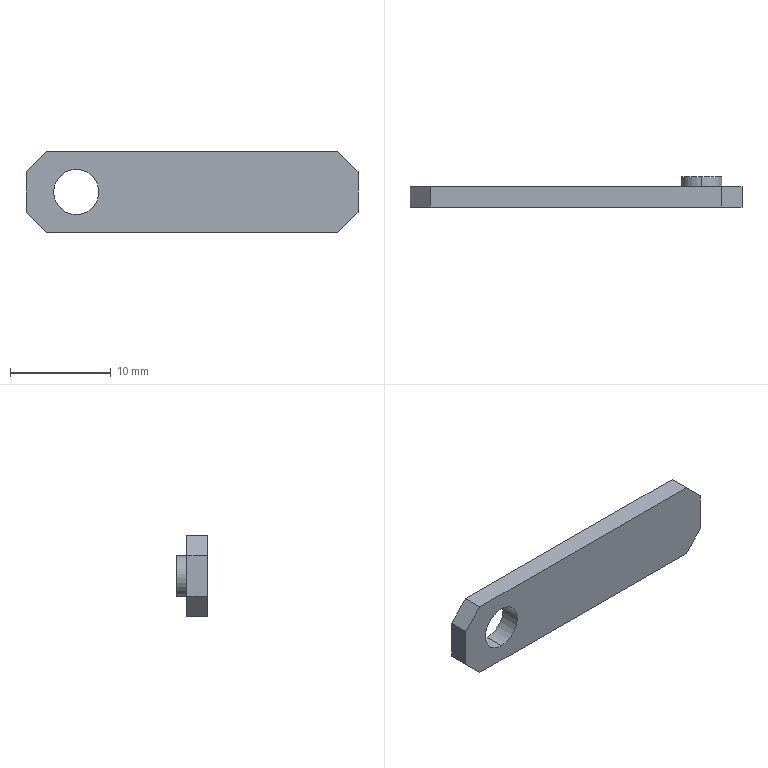Part | SolidWorks | features Chamfer 2, ICE 2, Extrusion 1 | 1 solid | 15 faces | box 33 x 3 x 8 mm | volume 492.758 mm3 | plane 11 | cylinder 4 | commonest cylinder face diameters 4 x2 4.5 x2
STEP:
#1=CARTESIAN_POINT('',(19.307,3.,-1.484));
#2=VERTEX_POINT('',#1);
#3=CARTESIAN_POINT('',(19.307,3.,-5.484));
#4=VERTEX_POINT('',#3);
#5=CARTESIAN_POINT('',(19.307,3.,-3.484));
#6=DIRECTION('',(0.,1.,0.));
#7=DIRECTION('',(0.,0.,1.));
#8=AXIS2_PLACEMENT_3D('',#5,#6,#7);
#9=CIRCLE('',#8,2.);
#10=EDGE_CURVE('',#2,#4,#9,.T.);
#11=ORIENTED_EDGE('',*,*,#10,.F.);
#12=CARTESIAN_POINT('',(19.307,2.,-1.484));
#13=VERTEX_POINT('',#12);
#14=CARTESIAN_POINT('',(19.307,3.,-1.484));
#15=DIRECTION('',(0.,-1.,0.));
#16=VECTOR('',#15,1000.);
#17=LINE('',#14,#16);
#18=EDGE_CURVE('',#2,#13,#17,.T.);
#19=ORIENTED_EDGE('',*,*,#18,.T.);
#20=CARTESIAN_POINT('',(19.307,2.,-5.484));
#21=VERTEX_POINT('',#20);
#22=CARTESIAN_POINT('',(19.307,2.,-3.484));
#23=DIRECTION('',(0.,1.,0.));
#24=DIRECTION('',(0.,0.,1.));
#25=AXIS2_PLACEMENT_3D('',#22,#23,#24);
#26=CIRCLE('',#25,2.);
#27=EDGE_CURVE('',#13,#21,#26,.T.);
#28=ORIENTED_EDGE('',*,*,#27,.T.);
#29=CARTESIAN_POINT('',(19.307,3.,-5.484));
#30=DIRECTION('',(0.,-1.,0.));
#31=VECTOR('',#30,1000.);
#32=LINE('',#29,#31);
#33=EDGE_CURVE('',#4,#21,#32,.T.);
#34=ORIENTED_EDGE('',*,*,#33,.F.);
#35=EDGE_LOOP('',(#11,#19,#28,#34));
#36=FACE_OUTER_BOUND('',#35,.T.);
#37=CARTESIAN_POINT('',(19.307,3.,-3.484));
#38=DIRECTION('',(0.,-1.,0.));
#39=DIRECTION('',(0.,0.,-1.));
#40=AXIS2_PLACEMENT_3D('',#37,#38,#39);
#41=CYLINDRICAL_SURFACE('',#40,2.);
#42=ADVANCED_FACE('',(#36),#41,.T.);
#43=CARTESIAN_POINT('',(-4.693,0.,-5.734));
#44=VERTEX_POINT('',#43);
#45=CARTESIAN_POINT('',(-4.693,0.,-1.234));
#46=VERTEX_POINT('',#45);
#47=CARTESIAN_POINT('',(-4.693,0.,-3.484));
#48=DIRECTION('',(0.,1.,0.));
#49=DIRECTION('',(0.,0.,1.));
#50=AXIS2_PLACEMENT_3D('',#47,#48,#49);
#51=CIRCLE('',#50,2.25);
#52=EDGE_CURVE('',#44,#46,#51,.T.);
#53=ORIENTED_EDGE('',*,*,#52,.F.);
#54=CARTESIAN_POINT('',(-4.693,2.,-5.734));
#55=VERTEX_POINT('',#54);
#56=CARTESIAN_POINT('',(-4.693,0.,-5.734));
#57=DIRECTION('',(0.,1.,0.));
#58=VECTOR('',#57,1000.);
#59=LINE('',#56,#58);
#60=EDGE_CURVE('',#44,#55,#59,.T.);
#61=ORIENTED_EDGE('',*,*,#60,.T.);
#62=CARTESIAN_POINT('',(-4.693,2.,-1.234));
#63=VERTEX_POINT('',#62);
#64=CARTESIAN_POINT('',(-4.693,2.,-3.484));
#65=DIRECTION('',(0.,1.,0.));
#66=DIRECTION('',(0.,0.,1.));
#67=AXIS2_PLACEMENT_3D('',#64,#65,#66);
#68=CIRCLE('',#67,2.25);
#69=EDGE_CURVE('',#55,#63,#68,.T.);
#70=ORIENTED_EDGE('',*,*,#69,.T.);
#71=CARTESIAN_POINT('',(-4.693,0.,-1.234));
#72=DIRECTION('',(0.,1.,0.));
#73=VECTOR('',#72,1000.);
#74=LINE('',#71,#73);
#75=EDGE_CURVE('',#46,#63,#74,.T.);
#76=ORIENTED_EDGE('',*,*,#75,.F.);
#77=EDGE_LOOP('',(#53,#61,#70,#76));
#78=FACE_OUTER_BOUND('',#77,.T.);
#79=CARTESIAN_POINT('',(-4.693,0.,-3.484));
#80=DIRECTION('',(0.,1.,0.));
#81=DIRECTION('',(0.,0.,1.));
#82=AXIS2_PLACEMENT_3D('',#79,#80,#81);
#83=CYLINDRICAL_SURFACE('',#82,2.25);
#84=ADVANCED_FACE('',(#78),#83,.F.);
#85=CARTESIAN_POINT('',(23.307,2.,-1.484));
#86=VERTEX_POINT('',#85);
#87=CARTESIAN_POINT('',(23.307,2.,-5.484));
#88=VERTEX_POINT('',#87);
#89=CARTESIAN_POINT('',(23.307,2.,-7.484));
#90=DIRECTION('',(0.,0.,-1.));
#91=VECTOR('',#90,1000.);
#92=LINE('',#89,#91);
#93=EDGE_CURVE('',#86,#88,#92,.T.);
#94=ORIENTED_EDGE('',*,*,#93,.T.);
#95=CARTESIAN_POINT('',(21.307,2.,-7.484));
#96=VERTEX_POINT('',#95);
#97=CARTESIAN_POINT('',(14.396,2.,-14.396));
#98=DIRECTION('',(-0.7071,0.,-0.7071));
#99=VECTOR('',#98,1000.);
#100=LINE('',#97,#99);
#101=EDGE_CURVE('',#88,#96,#100,.T.);
#102=ORIENTED_EDGE('',*,*,#101,.T.);
#103=CARTESIAN_POINT('',(-7.693,2.,-7.484));
#104=VERTEX_POINT('',#103);
#105=CARTESIAN_POINT('',(-9.693,2.,-7.484));
#106=DIRECTION('',(-1.,0.,0.));
#107=VECTOR('',#106,1000.);
#108=LINE('',#105,#107);
#109=EDGE_CURVE('',#96,#104,#108,.T.);
#110=ORIENTED_EDGE('',*,*,#109,.T.);
#111=CARTESIAN_POINT('',(-9.693,2.,-5.484));
#112=VERTEX_POINT('',#111);
#113=CARTESIAN_POINT('',(-7.589,2.,-7.589));
#114=DIRECTION('',(-0.7071,0.,0.7071));
#115=VECTOR('',#114,1000.);
#116=LINE('',#113,#115);
#117=EDGE_CURVE('',#104,#112,#116,.T.);
#118=ORIENTED_EDGE('',*,*,#117,.T.);
#119=CARTESIAN_POINT('',(-9.693,2.,-1.484));
#120=VERTEX_POINT('',#119);
#121=CARTESIAN_POINT('',(-9.693,2.,-7.484));
#122=DIRECTION('',(0.,0.,1.));
#123=VECTOR('',#122,1000.);
#124=LINE('',#121,#123);
#125=EDGE_CURVE('',#112,#120,#124,.T.);
#126=ORIENTED_EDGE('',*,*,#125,.T.);
#127=CARTESIAN_POINT('',(-7.693,2.,0.5156));
#128=VERTEX_POINT('',#127);
#129=CARTESIAN_POINT('',(-4.104,2.,4.104));
#130=DIRECTION('',(0.7071,0.,0.7071));
#131=VECTOR('',#130,1000.);
#132=LINE('',#129,#131);
#133=EDGE_CURVE('',#120,#128,#132,.T.);
#134=ORIENTED_EDGE('',*,*,#133,.T.);
#135=CARTESIAN_POINT('',(21.307,2.,0.5156));
#136=VERTEX_POINT('',#135);
#137=CARTESIAN_POINT('',(-9.693,2.,0.5156));
#138=DIRECTION('',(1.,0.,0.));
#139=VECTOR('',#138,1000.);
#140=LINE('',#137,#139);
#141=EDGE_CURVE('',#128,#136,#140,.T.);
#142=ORIENTED_EDGE('',*,*,#141,.T.);
#143=CARTESIAN_POINT('',(10.911,2.,10.911));
#144=DIRECTION('',(0.7071,0.,-0.7071));
#145=VECTOR('',#144,1000.);
#146=LINE('',#143,#145);
#147=EDGE_CURVE('',#136,#86,#146,.T.);
#148=ORIENTED_EDGE('',*,*,#147,.T.);
#149=EDGE_LOOP('',(#94,#102,#110,#118,#126,#134,#142,#148));
#150=FACE_OUTER_BOUND('',#149,.T.);
#151=CARTESIAN_POINT('',(-4.693,2.,-3.484));
#152=DIRECTION('',(0.,1.,0.));
#153=DIRECTION('',(0.,0.,1.));
#154=AXIS2_PLACEMENT_3D('',#151,#152,#153);
#155=CIRCLE('',#154,2.25);
#156=EDGE_CURVE('',#63,#55,#155,.T.);
#157=ORIENTED_EDGE('',*,*,#156,.F.);
#158=ORIENTED_EDGE('',*,*,#69,.F.);
#159=EDGE_LOOP('',(#157,#158));
#160=FACE_BOUND('',#159,.T.);
#161=CARTESIAN_POINT('',(19.307,2.,-3.484));
#162=DIRECTION('',(0.,1.,0.));
#163=DIRECTION('',(0.,0.,1.));
#164=AXIS2_PLACEMENT_3D('',#161,#162,#163);
#165=CIRCLE('',#164,2.);
#166=EDGE_CURVE('',#21,#13,#165,.T.);
#167=ORIENTED_EDGE('',*,*,#166,.F.);
#168=ORIENTED_EDGE('',*,*,#27,.F.);
#169=EDGE_LOOP('',(#167,#168));
#170=FACE_BOUND('',#169,.T.);
#171=CARTESIAN_POINT('',(0.,2.,0.));
#172=DIRECTION('',(0.,1.,0.));
#173=DIRECTION('',(0.,0.,1.));
#174=AXIS2_PLACEMENT_3D('',#171,#172,#173);
#175=PLANE('',#174);
#176=ADVANCED_FACE('',(#150,#160,#170),#175,.T.);
#177=CARTESIAN_POINT('',(-9.693,0.,-5.484));
#178=VERTEX_POINT('',#177);
#179=CARTESIAN_POINT('',(-9.693,0.,-1.484));
#180=VERTEX_POINT('',#179);
#181=CARTESIAN_POINT('',(-9.693,0.,-7.484));
#182=DIRECTION('',(0.,0.,1.));
#183=VECTOR('',#182,1000.);
#184=LINE('',#181,#183);
#185=EDGE_CURVE('',#178,#180,#184,.T.);
#186=ORIENTED_EDGE('',*,*,#185,.T.);
#187=CARTESIAN_POINT('',(-9.693,2.,-1.484));
#188=DIRECTION('',(0.,1.,0.));
#189=VECTOR('',#188,1000.);
#190=LINE('',#187,#189);
#191=EDGE_CURVE('',#180,#120,#190,.T.);
#192=ORIENTED_EDGE('',*,*,#191,.T.);
#193=ORIENTED_EDGE('',*,*,#125,.F.);
#194=CARTESIAN_POINT('',(-9.693,2.,-5.484));
#195=DIRECTION('',(0.,-1.,0.));
#196=VECTOR('',#195,1000.);
#197=LINE('',#194,#196);
#198=EDGE_CURVE('',#112,#178,#197,.T.);
#199=ORIENTED_EDGE('',*,*,#198,.T.);
#200=EDGE_LOOP('',(#186,#192,#193,#199));
#201=FACE_OUTER_BOUND('',#200,.T.);
#202=CARTESIAN_POINT('',(-9.693,2.,-7.484));
#203=DIRECTION('',(1.,0.,0.));
#204=DIRECTION('',(0.,0.,-1.));
#205=AXIS2_PLACEMENT_3D('',#202,#203,#204);
#206=PLANE('',#205);
#207=ADVANCED_FACE('',(#201),#206,.F.);
#208=CARTESIAN_POINT('',(-7.693,0.,0.5156));
#209=VERTEX_POINT('',#208);
#210=CARTESIAN_POINT('',(21.307,0.,0.5156));
#211=VERTEX_POINT('',#210);
#212=CARTESIAN_POINT('',(-9.693,0.,0.5156));
#213=DIRECTION('',(1.,0.,0.));
#214=VECTOR('',#213,1000.);
#215=LINE('',#212,#214);
#216=EDGE_CURVE('',#209,#211,#215,.T.);
#217=ORIENTED_EDGE('',*,*,#216,.T.);
#218=CARTESIAN_POINT('',(21.307,2.,0.5156));
#219=DIRECTION('',(0.,1.,0.));
#220=VECTOR('',#219,1000.);
#221=LINE('',#218,#220);
#222=EDGE_CURVE('',#211,#136,#221,.T.);
#223=ORIENTED_EDGE('',*,*,#222,.T.);
#224=ORIENTED_EDGE('',*,*,#141,.F.);
#225=CARTESIAN_POINT('',(-7.693,2.,0.5156));
#226=DIRECTION('',(0.,-1.,0.));
#227=VECTOR('',#226,1000.);
#228=LINE('',#225,#227);
#229=EDGE_CURVE('',#128,#209,#228,.T.);
#230=ORIENTED_EDGE('',*,*,#229,.T.);
#231=EDGE_LOOP('',(#217,#223,#224,#230));
#232=FACE_OUTER_BOUND('',#231,.T.);
#233=CARTESIAN_POINT('',(-9.693,2.,0.5156));
#234=DIRECTION('',(0.,0.,-1.));
#235=DIRECTION('',(-1.,0.,0.));
#236=AXIS2_PLACEMENT_3D('',#233,#234,#235);
#237=PLANE('',#236);
#238=ADVANCED_FACE('',(#232),#237,.F.);
#239=CARTESIAN_POINT('',(23.307,0.,-1.484));
#240=VERTEX_POINT('',#239);
#241=CARTESIAN_POINT('',(23.307,0.,-5.484));
#242=VERTEX_POINT('',#241);
#243=CARTESIAN_POINT('',(23.307,0.,-7.484));
#244=DIRECTION('',(0.,0.,-1.));
#245=VECTOR('',#244,1000.);
#246=LINE('',#243,#245);
#247=EDGE_CURVE('',#240,#242,#246,.T.);
#248=ORIENTED_EDGE('',*,*,#247,.T.);
#249=CARTESIAN_POINT('',(23.307,2.,-5.484));
#250=DIRECTION('',(0.,1.,0.));
#251=VECTOR('',#250,1000.);
#252=LINE('',#249,#251);
#253=EDGE_CURVE('',#242,#88,#252,.T.);
#254=ORIENTED_EDGE('',*,*,#253,.T.);
#255=ORIENTED_EDGE('',*,*,#93,.F.);
#256=CARTESIAN_POINT('',(23.307,2.,-1.484));
#257=DIRECTION('',(0.,-1.,0.));
#258=VECTOR('',#257,1000.);
#259=LINE('',#256,#258);
#260=EDGE_CURVE('',#86,#240,#259,.T.);
#261=ORIENTED_EDGE('',*,*,#260,.T.);
#262=EDGE_LOOP('',(#248,#254,#255,#261));
#263=FACE_OUTER_BOUND('',#262,.T.);
#264=CARTESIAN_POINT('',(23.307,2.,-7.484));
#265=DIRECTION('',(-1.,0.,0.));
#266=DIRECTION('',(0.,0.,1.));
#267=AXIS2_PLACEMENT_3D('',#264,#265,#266);
#268=PLANE('',#267);
#269=ADVANCED_FACE('',(#263),#268,.F.);
#270=ORIENTED_EDGE('',*,*,#109,.F.);
#271=CARTESIAN_POINT('',(21.307,0.,-7.484));
#272=VERTEX_POINT('',#271);
#273=CARTESIAN_POINT('',(21.307,2.,-7.484));
#274=DIRECTION('',(0.,-1.,0.));
#275=VECTOR('',#274,1000.);
#276=LINE('',#273,#275);
#277=EDGE_CURVE('',#96,#272,#276,.T.);
#278=ORIENTED_EDGE('',*,*,#277,.T.);
#279=CARTESIAN_POINT('',(-7.693,0.,-7.484));
#280=VERTEX_POINT('',#279);
#281=CARTESIAN_POINT('',(-9.693,0.,-7.484));
#282=DIRECTION('',(-1.,0.,0.));
#283=VECTOR('',#282,1000.);
#284=LINE('',#281,#283);
#285=EDGE_CURVE('',#272,#280,#284,.T.);
#286=ORIENTED_EDGE('',*,*,#285,.T.);
#287=CARTESIAN_POINT('',(-7.693,2.,-7.484));
#288=DIRECTION('',(0.,1.,0.));
#289=VECTOR('',#288,1000.);
#290=LINE('',#287,#289);
#291=EDGE_CURVE('',#280,#104,#290,.T.);
#292=ORIENTED_EDGE('',*,*,#291,.T.);
#293=EDGE_LOOP('',(#270,#278,#286,#292));
#294=FACE_OUTER_BOUND('',#293,.T.);
#295=CARTESIAN_POINT('',(-9.693,2.,-7.484));
#296=DIRECTION('',(0.,0.,1.));
#297=DIRECTION('',(1.,0.,0.));
#298=AXIS2_PLACEMENT_3D('',#295,#296,#297);
#299=PLANE('',#298);
#300=ADVANCED_FACE('',(#294),#299,.F.);
#301=CARTESIAN_POINT('',(-4.693,0.,-3.484));
#302=DIRECTION('',(0.,1.,0.));
#303=DIRECTION('',(0.,0.,1.));
#304=AXIS2_PLACEMENT_3D('',#301,#302,#303);
#305=CIRCLE('',#304,2.25);
#306=EDGE_CURVE('',#46,#44,#305,.T.);
#307=ORIENTED_EDGE('',*,*,#306,.T.);
#308=ORIENTED_EDGE('',*,*,#52,.T.);
#309=EDGE_LOOP('',(#307,#308));
#310=FACE_BOUND('',#309,.T.);
#311=ORIENTED_EDGE('',*,*,#285,.F.);
#312=CARTESIAN_POINT('',(21.307,0.,-7.484));
#313=DIRECTION('',(0.7071,0.,0.7071));
#314=VECTOR('',#313,1000.);
#315=LINE('',#312,#314);
#316=EDGE_CURVE('',#272,#242,#315,.T.);
#317=ORIENTED_EDGE('',*,*,#316,.T.);
#318=ORIENTED_EDGE('',*,*,#247,.F.);
#319=CARTESIAN_POINT('',(23.307,0.,-1.484));
#320=DIRECTION('',(-0.7071,0.,0.7071));
#321=VECTOR('',#320,1000.);
#322=LINE('',#319,#321);
#323=EDGE_CURVE('',#240,#211,#322,.T.);
#324=ORIENTED_EDGE('',*,*,#323,.T.);
#325=ORIENTED_EDGE('',*,*,#216,.F.);
#326=CARTESIAN_POINT('',(-7.693,0.,0.5156));
#327=DIRECTION('',(-0.7071,0.,-0.7071));
#328=VECTOR('',#327,1000.);
#329=LINE('',#326,#328);
#330=EDGE_CURVE('',#209,#180,#329,.T.);
#331=ORIENTED_EDGE('',*,*,#330,.T.);
#332=ORIENTED_EDGE('',*,*,#185,.F.);
#333=CARTESIAN_POINT('',(-9.693,0.,-5.484));
#334=DIRECTION('',(0.7071,0.,-0.7071));
#335=VECTOR('',#334,1000.);
#336=LINE('',#333,#335);
#337=EDGE_CURVE('',#178,#280,#336,.T.);
#338=ORIENTED_EDGE('',*,*,#337,.T.);
#339=EDGE_LOOP('',(#311,#317,#318,#324,#325,#331,#332,#338));
#340=FACE_OUTER_BOUND('',#339,.T.);
#341=CARTESIAN_POINT('',(0.,0.,0.));
#342=DIRECTION('',(0.,1.,0.));
#343=DIRECTION('',(0.,0.,1.));
#344=AXIS2_PLACEMENT_3D('',#341,#342,#343);
#345=PLANE('',#344);
#346=ADVANCED_FACE('',(#310,#340),#345,.F.);
#347=ORIENTED_EDGE('',*,*,#60,.F.);
#348=ORIENTED_EDGE('',*,*,#306,.F.);
#349=ORIENTED_EDGE('',*,*,#75,.T.);
#350=ORIENTED_EDGE('',*,*,#156,.T.);
#351=EDGE_LOOP('',(#347,#348,#349,#350));
#352=FACE_OUTER_BOUND('',#351,.T.);
#353=CARTESIAN_POINT('',(-4.693,0.,-3.484));
#354=DIRECTION('',(0.,1.,0.));
#355=DIRECTION('',(0.,0.,1.));
#356=AXIS2_PLACEMENT_3D('',#353,#354,#355);
#357=CYLINDRICAL_SURFACE('',#356,2.25);
#358=ADVANCED_FACE('',(#352),#357,.F.);
#359=ORIENTED_EDGE('',*,*,#18,.F.);
#360=CARTESIAN_POINT('',(19.307,3.,-3.484));
#361=DIRECTION('',(0.,1.,0.));
#362=DIRECTION('',(0.,0.,1.));
#363=AXIS2_PLACEMENT_3D('',#360,#361,#362);
#364=CIRCLE('',#363,2.);
#365=EDGE_CURVE('',#4,#2,#364,.T.);
#366=ORIENTED_EDGE('',*,*,#365,.F.);
#367=ORIENTED_EDGE('',*,*,#33,.T.);
#368=ORIENTED_EDGE('',*,*,#166,.T.);
#369=EDGE_LOOP('',(#359,#366,#367,#368));
#370=FACE_OUTER_BOUND('',#369,.T.);
#371=CARTESIAN_POINT('',(19.307,3.,-3.484));
#372=DIRECTION('',(0.,-1.,0.));
#373=DIRECTION('',(0.,0.,-1.));
#374=AXIS2_PLACEMENT_3D('',#371,#372,#373);
#375=CYLINDRICAL_SURFACE('',#374,2.);
#376=ADVANCED_FACE('',(#370),#375,.T.);
#377=ORIENTED_EDGE('',*,*,#365,.T.);
#378=ORIENTED_EDGE('',*,*,#10,.T.);
#379=EDGE_LOOP('',(#377,#378));
#380=FACE_OUTER_BOUND('',#379,.T.);
#381=CARTESIAN_POINT('',(19.307,3.,-3.484));
#382=DIRECTION('',(0.,1.,0.));
#383=DIRECTION('',(0.,0.,1.));
#384=AXIS2_PLACEMENT_3D('',#381,#382,#383);
#385=PLANE('',#384);
#386=ADVANCED_FACE('',(#380),#385,.T.);
#387=ORIENTED_EDGE('',*,*,#101,.F.);
#388=ORIENTED_EDGE('',*,*,#253,.F.);
#389=ORIENTED_EDGE('',*,*,#316,.F.);
#390=ORIENTED_EDGE('',*,*,#277,.F.);
#391=EDGE_LOOP('',(#387,#388,#389,#390));
#392=FACE_OUTER_BOUND('',#391,.T.);
#393=CARTESIAN_POINT('',(21.307,2.,-7.484));
#394=DIRECTION('',(-0.7071,0.,0.7071));
#395=DIRECTION('',(0.,-1.,0.));
#396=AXIS2_PLACEMENT_3D('',#393,#394,#395);
#397=PLANE('',#396);
#398=ADVANCED_FACE('',(#392),#397,.F.);
#399=ORIENTED_EDGE('',*,*,#147,.F.);
#400=ORIENTED_EDGE('',*,*,#222,.F.);
#401=ORIENTED_EDGE('',*,*,#323,.F.);
#402=ORIENTED_EDGE('',*,*,#260,.F.);
#403=EDGE_LOOP('',(#399,#400,#401,#402));
#404=FACE_OUTER_BOUND('',#403,.T.);
#405=CARTESIAN_POINT('',(23.307,2.,-1.484));
#406=DIRECTION('',(-0.7071,0.,-0.7071));
#407=DIRECTION('',(0.,-1.,0.));
#408=AXIS2_PLACEMENT_3D('',#405,#406,#407);
#409=PLANE('',#408);
#410=ADVANCED_FACE('',(#404),#409,.F.);
#411=ORIENTED_EDGE('',*,*,#133,.F.);
#412=ORIENTED_EDGE('',*,*,#191,.F.);
#413=ORIENTED_EDGE('',*,*,#330,.F.);
#414=ORIENTED_EDGE('',*,*,#229,.F.);
#415=EDGE_LOOP('',(#411,#412,#413,#414));
#416=FACE_OUTER_BOUND('',#415,.T.);
#417=CARTESIAN_POINT('',(-7.693,2.,0.5156));
#418=DIRECTION('',(0.7071,0.,-0.7071));
#419=DIRECTION('',(0.,-1.,0.));
#420=AXIS2_PLACEMENT_3D('',#417,#418,#419);
#421=PLANE('',#420);
#422=ADVANCED_FACE('',(#416),#421,.F.);
#423=ORIENTED_EDGE('',*,*,#117,.F.);
#424=ORIENTED_EDGE('',*,*,#291,.F.);
#425=ORIENTED_EDGE('',*,*,#337,.F.);
#426=ORIENTED_EDGE('',*,*,#198,.F.);
#427=EDGE_LOOP('',(#423,#424,#425,#426));
#428=FACE_OUTER_BOUND('',#427,.T.);
#429=CARTESIAN_POINT('',(-9.693,2.,-5.484));
#430=DIRECTION('',(0.7071,0.,0.7071));
#431=DIRECTION('',(0.,-1.,0.));
#432=AXIS2_PLACEMENT_3D('',#429,#430,#431);
#433=PLANE('',#432);
#434=ADVANCED_FACE('',(#428),#433,.F.);
#435=CLOSED_SHELL('',(#42,#84,#176,#207,#238,#269,#300,#346,#358,#376,#386,#398,#410,#422,#434));
#436=MANIFOLD_SOLID_BREP('',#435);
#437=CARTESIAN_POINT('',(0.,0.,0.));
#438=DIRECTION('',(0.,0.,1.));
#439=DIRECTION('',(1.,0.,0.));
#440=AXIS2_PLACEMENT_3D('',#437,#438,#439);
#441=(LENGTH_UNIT()NAMED_UNIT(*)SI_UNIT(.MILLI.,.METRE.));
#442=UNCERTAINTY_MEASURE_WITH_UNIT(LENGTH_MEASURE(0.00001),#441,'','');
#443=(NAMED_UNIT(*)PLANE_ANGLE_UNIT()SI_UNIT($,.RADIAN.));
#444=(NAMED_UNIT(*)SI_UNIT($,.STERADIAN.)SOLID_ANGLE_UNIT());
#445=(GEOMETRIC_REPRESENTATION_CONTEXT(3)GLOBAL_UNCERTAINTY_ASSIGNED_CONTEXT((#442))GLOBAL_UNIT_ASSIGNED_CONTEXT((#441,#443,#444))REPRESENTATION_CONTEXT('',''));
#446=ADVANCED_BREP_SHAPE_REPRESENTATION('',(#436,#440),#445);